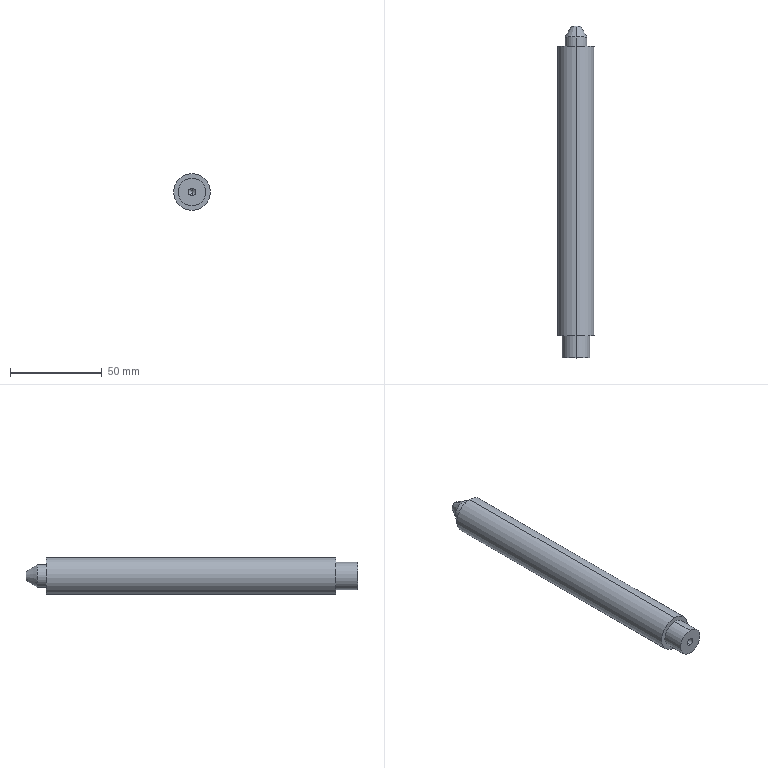Part | STEP file | 1 solid | 16 faces | box 20 x 181 x 20 mm | volume 52508 mm3 | cylinder 8 | cone 4 | plane 4 | commonest cylinder face diameters 4.2 x2 12 x2 15 x2 20 x2
STEP:
#1=CARTESIAN_POINT('',(0.,0.,0.));
#2=DIRECTION('',(0.,0.,1.));
#3=DIRECTION('',(1.,0.,0.));
#4=AXIS2_PLACEMENT_3D('',#1,#2,#3);
#5=CARTESIAN_POINT('',(0.,12.4,-2.1));
#6=VERTEX_POINT('',#5);
#7=CARTESIAN_POINT('',(0.,0.,-2.1));
#8=VERTEX_POINT('',#7);
#9=CARTESIAN_POINT('',(0.,0.,-2.1));
#10=DIRECTION('',(0.,-1.,0.));
#11=VECTOR('',#10,1.);
#12=LINE('',#9,#11);
#13=CARTESIAN_POINT('',(0.,0.,0.));
#14=DIRECTION('',(0.,-1.,0.));
#15=DIRECTION('',(0.,0.,-1.));
#16=AXIS2_PLACEMENT_3D('',#13,#14,#15);
#17=CYLINDRICAL_SURFACE('',#16,2.1);
#18=CARTESIAN_POINT('',(6.283,0.));
#19=DIRECTION('',(0.,1.));
#20=VECTOR('',#19,1.);
#21=LINE('',#18,#20);
#22=(GEOMETRIC_REPRESENTATION_CONTEXT(2)PARAMETRIC_REPRESENTATION_CONTEXT()REPRESENTATION_CONTEXT('',''));
#23=DEFINITIONAL_REPRESENTATION('',(#21),#22);
#24=PCURVE('',#17,#23);
#25=CARTESIAN_POINT('',(0.,0.,0.));
#26=DIRECTION('',(0.,-1.,0.));
#27=DIRECTION('',(0.,0.,-1.));
#28=AXIS2_PLACEMENT_3D('',#25,#26,#27);
#29=CYLINDRICAL_SURFACE('',#28,2.1);
#30=CARTESIAN_POINT('',(0.,0.));
#31=DIRECTION('',(0.,1.));
#32=VECTOR('',#31,1.);
#33=LINE('',#30,#32);
#34=(GEOMETRIC_REPRESENTATION_CONTEXT(2)PARAMETRIC_REPRESENTATION_CONTEXT()REPRESENTATION_CONTEXT('',''));
#35=DEFINITIONAL_REPRESENTATION('',(#33),#34);
#36=PCURVE('',#29,#35);
#37=SURFACE_CURVE('',#12,(#24,#36),.PCURVE_S1.);
#38=EDGE_CURVE('',#6,#8,#37,.T.);
#39=ORIENTED_EDGE('',*,*,#38,.T.);
#40=CARTESIAN_POINT('',(0.,0.,2.1));
#41=VERTEX_POINT('',#40);
#42=CARTESIAN_POINT('',(0.,0.,0.));
#43=DIRECTION('',(0.,-1.,0.));
#44=DIRECTION('',(0.,0.,-1.));
#45=AXIS2_PLACEMENT_3D('',#42,#43,#44);
#46=CIRCLE('',#45,2.1);
#47=CARTESIAN_POINT('',(0.,0.));
#48=DIRECTION('',(1.,0.));
#49=VECTOR('',#48,1.);
#50=LINE('',#47,#49);
#51=(GEOMETRIC_REPRESENTATION_CONTEXT(2)PARAMETRIC_REPRESENTATION_CONTEXT()REPRESENTATION_CONTEXT('',''));
#52=DEFINITIONAL_REPRESENTATION('',(#50),#51);
#53=PCURVE('',#17,#52);
#54=CARTESIAN_POINT('',(0.,0.,0.));
#55=DIRECTION('',(0.,-1.,0.));
#56=DIRECTION('',(0.,0.,-1.));
#57=AXIS2_PLACEMENT_3D('',#54,#55,#56);
#58=PLANE('',#57);
#59=CARTESIAN_POINT('',(0.,0.));
#60=DIRECTION('',(1.,0.));
#61=AXIS2_PLACEMENT_2D('',#59,#60);
#62=CIRCLE('',#61,2.1);
#63=(GEOMETRIC_REPRESENTATION_CONTEXT(2)PARAMETRIC_REPRESENTATION_CONTEXT()REPRESENTATION_CONTEXT('',''));
#64=DEFINITIONAL_REPRESENTATION('',(#62),#63);
#65=PCURVE('',#58,#64);
#66=SURFACE_CURVE('',#46,(#53,#65),.PCURVE_S1.);
#67=EDGE_CURVE('',#41,#8,#66,.T.);
#68=ORIENTED_EDGE('',*,*,#67,.F.);
#69=CARTESIAN_POINT('',(0.,12.4,2.1));
#70=VERTEX_POINT('',#69);
#71=CARTESIAN_POINT('',(0.,0.,2.1));
#72=DIRECTION('',(0.,-1.,0.));
#73=VECTOR('',#72,1.);
#74=LINE('',#71,#73);
#75=CARTESIAN_POINT('',(3.142,0.));
#76=DIRECTION('',(0.,1.));
#77=VECTOR('',#76,1.);
#78=LINE('',#75,#77);
#79=(GEOMETRIC_REPRESENTATION_CONTEXT(2)PARAMETRIC_REPRESENTATION_CONTEXT()REPRESENTATION_CONTEXT('',''));
#80=DEFINITIONAL_REPRESENTATION('',(#78),#79);
#81=PCURVE('',#17,#80);
#82=CARTESIAN_POINT('',(3.142,0.));
#83=DIRECTION('',(0.,1.));
#84=VECTOR('',#83,1.);
#85=LINE('',#82,#84);
#86=(GEOMETRIC_REPRESENTATION_CONTEXT(2)PARAMETRIC_REPRESENTATION_CONTEXT()REPRESENTATION_CONTEXT('',''));
#87=DEFINITIONAL_REPRESENTATION('',(#85),#86);
#88=PCURVE('',#29,#87);
#89=SURFACE_CURVE('',#74,(#81,#88),.PCURVE_S1.);
#90=EDGE_CURVE('',#70,#41,#89,.T.);
#91=ORIENTED_EDGE('',*,*,#90,.F.);
#92=CARTESIAN_POINT('',(0.,12.4,0.));
#93=DIRECTION('',(0.,-1.,0.));
#94=DIRECTION('',(0.,0.,-1.));
#95=AXIS2_PLACEMENT_3D('',#92,#93,#94);
#96=CIRCLE('',#95,2.1);
#97=CARTESIAN_POINT('',(0.,-12.4));
#98=DIRECTION('',(1.,0.));
#99=VECTOR('',#98,1.);
#100=LINE('',#97,#99);
#101=(GEOMETRIC_REPRESENTATION_CONTEXT(2)PARAMETRIC_REPRESENTATION_CONTEXT()REPRESENTATION_CONTEXT('',''));
#102=DEFINITIONAL_REPRESENTATION('',(#100),#101);
#103=PCURVE('',#17,#102);
#104=CARTESIAN_POINT('',(0.,12.4,0.));
#105=DIRECTION('',(0.,-1.,0.));
#106=DIRECTION('',(0.,0.,-1.));
#107=AXIS2_PLACEMENT_3D('',#104,#105,#106);
#108=CONICAL_SURFACE('',#107,2.1,1.03);
#109=CARTESIAN_POINT('',(0.,0.));
#110=DIRECTION('',(1.,0.));
#111=VECTOR('',#110,1.);
#112=LINE('',#109,#111);
#113=(GEOMETRIC_REPRESENTATION_CONTEXT(2)PARAMETRIC_REPRESENTATION_CONTEXT()REPRESENTATION_CONTEXT('',''));
#114=DEFINITIONAL_REPRESENTATION('',(#112),#113);
#115=PCURVE('',#108,#114);
#116=SURFACE_CURVE('',#96,(#103,#115),.PCURVE_S1.);
#117=EDGE_CURVE('',#70,#6,#116,.T.);
#118=ORIENTED_EDGE('',*,*,#117,.T.);
#119=EDGE_LOOP('',(#39,#68,#91,#118));
#120=FACE_BOUND('',#119,.F.);
#121=ADVANCED_FACE('',(#120),#17,.F.);
#122=ORIENTED_EDGE('',*,*,#117,.F.);
#123=CARTESIAN_POINT('',(0.,13.662,0.));
#124=VERTEX_POINT('',#123);
#125=CARTESIAN_POINT('',(0.,12.4,2.1));
#126=DIRECTION('',(0.,-0.515,0.8572));
#127=VECTOR('',#126,1.);
#128=LINE('',#125,#127);
#129=CARTESIAN_POINT('',(3.142,0.));
#130=DIRECTION('',(0.,1.));
#131=VECTOR('',#130,1.);
#132=LINE('',#129,#131);
#133=(GEOMETRIC_REPRESENTATION_CONTEXT(2)PARAMETRIC_REPRESENTATION_CONTEXT()REPRESENTATION_CONTEXT('',''));
#134=DEFINITIONAL_REPRESENTATION('',(#132),#133);
#135=PCURVE('',#108,#134);
#136=CARTESIAN_POINT('',(0.,12.4,0.));
#137=DIRECTION('',(0.,-1.,0.));
#138=DIRECTION('',(0.,0.,-1.));
#139=AXIS2_PLACEMENT_3D('',#136,#137,#138);
#140=CONICAL_SURFACE('',#139,2.1,1.03);
#141=CARTESIAN_POINT('',(3.142,0.));
#142=DIRECTION('',(0.,1.));
#143=VECTOR('',#142,1.);
#144=LINE('',#141,#143);
#145=(GEOMETRIC_REPRESENTATION_CONTEXT(2)PARAMETRIC_REPRESENTATION_CONTEXT()REPRESENTATION_CONTEXT('',''));
#146=DEFINITIONAL_REPRESENTATION('',(#144),#145);
#147=PCURVE('',#140,#146);
#148=SURFACE_CURVE('',#128,(#135,#147),.PCURVE_S1.);
#149=EDGE_CURVE('',#124,#70,#148,.T.);
#150=ORIENTED_EDGE('',*,*,#149,.F.);
#151=CARTESIAN_POINT('',(0.,12.4,-2.1));
#152=DIRECTION('',(0.,-0.515,-0.8572));
#153=VECTOR('',#152,1.);
#154=LINE('',#151,#153);
#155=CARTESIAN_POINT('',(6.283,0.));
#156=DIRECTION('',(0.,1.));
#157=VECTOR('',#156,1.);
#158=LINE('',#155,#157);
#159=(GEOMETRIC_REPRESENTATION_CONTEXT(2)PARAMETRIC_REPRESENTATION_CONTEXT()REPRESENTATION_CONTEXT('',''));
#160=DEFINITIONAL_REPRESENTATION('',(#158),#159);
#161=PCURVE('',#108,#160);
#162=CARTESIAN_POINT('',(0.,0.));
#163=DIRECTION('',(0.,1.));
#164=VECTOR('',#163,1.);
#165=LINE('',#162,#164);
#166=(GEOMETRIC_REPRESENTATION_CONTEXT(2)PARAMETRIC_REPRESENTATION_CONTEXT()REPRESENTATION_CONTEXT('',''));
#167=DEFINITIONAL_REPRESENTATION('',(#165),#166);
#168=PCURVE('',#140,#167);
#169=SURFACE_CURVE('',#154,(#161,#168),.PCURVE_S1.);
#170=EDGE_CURVE('',#124,#6,#169,.T.);
#171=ORIENTED_EDGE('',*,*,#170,.T.);
#172=EDGE_LOOP('',(#122,#150,#171));
#173=FACE_BOUND('',#172,.F.);
#174=ADVANCED_FACE('',(#173),#108,.F.);
#175=CARTESIAN_POINT('',(0.,181.,-2.536));
#176=VERTEX_POINT('',#175);
#177=CARTESIAN_POINT('',(0.,181.,2.536));
#178=VERTEX_POINT('',#177);
#179=CARTESIAN_POINT('',(0.,181.,0.));
#180=DIRECTION('',(0.,-1.,0.));
#181=DIRECTION('',(0.,0.,-1.));
#182=AXIS2_PLACEMENT_3D('',#179,#180,#181);
#183=CIRCLE('',#182,2.536);
#184=CARTESIAN_POINT('',(0.,175.,0.));
#185=DIRECTION('',(0.,-1.,0.));
#186=DIRECTION('',(0.,0.,-1.));
#187=AXIS2_PLACEMENT_3D('',#184,#185,#186);
#188=CONICAL_SURFACE('',#187,6.,0.5236);
#189=CARTESIAN_POINT('',(0.,-6.));
#190=DIRECTION('',(1.,0.));
#191=VECTOR('',#190,1.);
#192=LINE('',#189,#191);
#193=(GEOMETRIC_REPRESENTATION_CONTEXT(2)PARAMETRIC_REPRESENTATION_CONTEXT()REPRESENTATION_CONTEXT('',''));
#194=DEFINITIONAL_REPRESENTATION('',(#192),#193);
#195=PCURVE('',#188,#194);
#196=CARTESIAN_POINT('',(2.536,181.,0.));
#197=DIRECTION('',(0.,1.,0.));
#198=DIRECTION('',(0.,0.,1.));
#199=AXIS2_PLACEMENT_3D('',#196,#197,#198);
#200=PLANE('',#199);
#201=CARTESIAN_POINT('',(-2.536,-2.536));
#202=CARTESIAN_POINT('',(-2.536,1.856));
#203=CARTESIAN_POINT('',(1.268,-0.3397));
#204=CARTESIAN_POINT('',(5.072,-2.536));
#205=CARTESIAN_POINT('',(1.268,-4.732));
#206=CARTESIAN_POINT('',(-2.536,-6.928));
#207=CARTESIAN_POINT('',(-2.536,-2.536));
#208=(BOUNDED_CURVE()B_SPLINE_CURVE(2,(#201,#202,#203,#204,#205,#206,#207),.UNSPECIFIED.,.T.,.F.)B_SPLINE_CURVE_WITH_KNOTS((1,2,2,2,2,1),(-2.094,0.,2.094,4.189,6.283,8.378),.UNSPECIFIED.)CURVE()GEOMETRIC_REPRESENTATION_ITEM()RATIONAL_B_SPLINE_CURVE((1.,0.5,1.,0.5,1.,0.5,1.))REPRESENTATION_ITEM(''));
#209=(GEOMETRIC_REPRESENTATION_CONTEXT(2)PARAMETRIC_REPRESENTATION_CONTEXT()REPRESENTATION_CONTEXT('',''));
#210=DEFINITIONAL_REPRESENTATION('',(#208),#209);
#211=PCURVE('',#200,#210);
#212=SURFACE_CURVE('',#183,(#195,#211),.PCURVE_S1.);
#213=EDGE_CURVE('',#176,#178,#212,.T.);
#214=ORIENTED_EDGE('',*,*,#213,.T.);
#215=CARTESIAN_POINT('',(0.,175.,6.));
#216=VERTEX_POINT('',#215);
#217=CARTESIAN_POINT('',(0.,175.,6.));
#218=DIRECTION('',(0.,-0.866,0.5));
#219=VECTOR('',#218,1.);
#220=LINE('',#217,#219);
#221=CARTESIAN_POINT('',(3.142,0.));
#222=DIRECTION('',(0.,1.));
#223=VECTOR('',#222,1.);
#224=LINE('',#221,#223);
#225=(GEOMETRIC_REPRESENTATION_CONTEXT(2)PARAMETRIC_REPRESENTATION_CONTEXT()REPRESENTATION_CONTEXT('',''));
#226=DEFINITIONAL_REPRESENTATION('',(#224),#225);
#227=PCURVE('',#188,#226);
#228=CARTESIAN_POINT('',(0.,175.,0.));
#229=DIRECTION('',(0.,-1.,0.));
#230=DIRECTION('',(0.,0.,-1.));
#231=AXIS2_PLACEMENT_3D('',#228,#229,#230);
#232=CONICAL_SURFACE('',#231,6.,0.5236);
#233=CARTESIAN_POINT('',(3.142,0.));
#234=DIRECTION('',(0.,1.));
#235=VECTOR('',#234,1.);
#236=LINE('',#233,#235);
#237=(GEOMETRIC_REPRESENTATION_CONTEXT(2)PARAMETRIC_REPRESENTATION_CONTEXT()REPRESENTATION_CONTEXT('',''));
#238=DEFINITIONAL_REPRESENTATION('',(#236),#237);
#239=PCURVE('',#232,#238);
#240=SURFACE_CURVE('',#220,(#227,#239),.PCURVE_S1.);
#241=EDGE_CURVE('',#178,#216,#240,.T.);
#242=ORIENTED_EDGE('',*,*,#241,.T.);
#243=CARTESIAN_POINT('',(0.,175.,-6.));
#244=VERTEX_POINT('',#243);
#245=CARTESIAN_POINT('',(0.,175.,0.));
#246=DIRECTION('',(0.,-1.,0.));
#247=DIRECTION('',(0.,0.,-1.));
#248=AXIS2_PLACEMENT_3D('',#245,#246,#247);
#249=CIRCLE('',#248,6.);
#250=CARTESIAN_POINT('',(0.,0.));
#251=DIRECTION('',(1.,0.));
#252=VECTOR('',#251,1.);
#253=LINE('',#250,#252);
#254=(GEOMETRIC_REPRESENTATION_CONTEXT(2)PARAMETRIC_REPRESENTATION_CONTEXT()REPRESENTATION_CONTEXT('',''));
#255=DEFINITIONAL_REPRESENTATION('',(#253),#254);
#256=PCURVE('',#188,#255);
#257=CARTESIAN_POINT('',(0.,0.,0.));
#258=DIRECTION('',(0.,-1.,0.));
#259=DIRECTION('',(0.,0.,-1.));
#260=AXIS2_PLACEMENT_3D('',#257,#258,#259);
#261=CYLINDRICAL_SURFACE('',#260,6.);
#262=CARTESIAN_POINT('',(0.,-175.));
#263=DIRECTION('',(1.,0.));
#264=VECTOR('',#263,1.);
#265=LINE('',#262,#264);
#266=(GEOMETRIC_REPRESENTATION_CONTEXT(2)PARAMETRIC_REPRESENTATION_CONTEXT()REPRESENTATION_CONTEXT('',''));
#267=DEFINITIONAL_REPRESENTATION('',(#265),#266);
#268=PCURVE('',#261,#267);
#269=SURFACE_CURVE('',#249,(#256,#268),.PCURVE_S1.);
#270=EDGE_CURVE('',#244,#216,#269,.T.);
#271=ORIENTED_EDGE('',*,*,#270,.F.);
#272=CARTESIAN_POINT('',(0.,175.,-6.));
#273=DIRECTION('',(0.,-0.866,-0.5));
#274=VECTOR('',#273,1.);
#275=LINE('',#272,#274);
#276=CARTESIAN_POINT('',(0.,0.));
#277=DIRECTION('',(0.,1.));
#278=VECTOR('',#277,1.);
#279=LINE('',#276,#278);
#280=(GEOMETRIC_REPRESENTATION_CONTEXT(2)PARAMETRIC_REPRESENTATION_CONTEXT()REPRESENTATION_CONTEXT('',''));
#281=DEFINITIONAL_REPRESENTATION('',(#279),#280);
#282=PCURVE('',#188,#281);
#283=CARTESIAN_POINT('',(6.283,0.));
#284=DIRECTION('',(0.,1.));
#285=VECTOR('',#284,1.);
#286=LINE('',#283,#285);
#287=(GEOMETRIC_REPRESENTATION_CONTEXT(2)PARAMETRIC_REPRESENTATION_CONTEXT()REPRESENTATION_CONTEXT('',''));
#288=DEFINITIONAL_REPRESENTATION('',(#286),#287);
#289=PCURVE('',#232,#288);
#290=SURFACE_CURVE('',#275,(#282,#289),.PCURVE_S1.);
#291=EDGE_CURVE('',#176,#244,#290,.T.);
#292=ORIENTED_EDGE('',*,*,#291,.F.);
#293=EDGE_LOOP('',(#214,#242,#271,#292));
#294=FACE_BOUND('',#293,.T.);
#295=ADVANCED_FACE('',(#294),#188,.T.);
#296=ORIENTED_EDGE('',*,*,#270,.T.);
#297=CARTESIAN_POINT('',(0.,170.,6.));
#298=VERTEX_POINT('',#297);
#299=CARTESIAN_POINT('',(0.,0.,6.));
#300=DIRECTION('',(0.,-1.,0.));
#301=VECTOR('',#300,1.);
#302=LINE('',#299,#301);
#303=CARTESIAN_POINT('',(3.142,0.));
#304=DIRECTION('',(0.,1.));
#305=VECTOR('',#304,1.);
#306=LINE('',#303,#305);
#307=(GEOMETRIC_REPRESENTATION_CONTEXT(2)PARAMETRIC_REPRESENTATION_CONTEXT()REPRESENTATION_CONTEXT('',''));
#308=DEFINITIONAL_REPRESENTATION('',(#306),#307);
#309=PCURVE('',#261,#308);
#310=CARTESIAN_POINT('',(0.,0.,0.));
#311=DIRECTION('',(0.,-1.,0.));
#312=DIRECTION('',(0.,0.,-1.));
#313=AXIS2_PLACEMENT_3D('',#310,#311,#312);
#314=CYLINDRICAL_SURFACE('',#313,6.);
#315=CARTESIAN_POINT('',(3.142,0.));
#316=DIRECTION('',(0.,1.));
#317=VECTOR('',#316,1.);
#318=LINE('',#315,#317);
#319=(GEOMETRIC_REPRESENTATION_CONTEXT(2)PARAMETRIC_REPRESENTATION_CONTEXT()REPRESENTATION_CONTEXT('',''));
#320=DEFINITIONAL_REPRESENTATION('',(#318),#319);
#321=PCURVE('',#314,#320);
#322=SURFACE_CURVE('',#302,(#309,#321),.PCURVE_S1.);
#323=EDGE_CURVE('',#216,#298,#322,.T.);
#324=ORIENTED_EDGE('',*,*,#323,.T.);
#325=CARTESIAN_POINT('',(0.,170.,-6.));
#326=VERTEX_POINT('',#325);
#327=CARTESIAN_POINT('',(0.,170.,0.));
#328=DIRECTION('',(0.,-1.,0.));
#329=DIRECTION('',(0.,0.,-1.));
#330=AXIS2_PLACEMENT_3D('',#327,#328,#329);
#331=CIRCLE('',#330,6.);
#332=CARTESIAN_POINT('',(0.,-170.));
#333=DIRECTION('',(1.,0.));
#334=VECTOR('',#333,1.);
#335=LINE('',#332,#334);
#336=(GEOMETRIC_REPRESENTATION_CONTEXT(2)PARAMETRIC_REPRESENTATION_CONTEXT()REPRESENTATION_CONTEXT('',''));
#337=DEFINITIONAL_REPRESENTATION('',(#335),#336);
#338=PCURVE('',#261,#337);
#339=CARTESIAN_POINT('',(10.,170.,0.));
#340=DIRECTION('',(0.,1.,0.));
#341=DIRECTION('',(0.,0.,1.));
#342=AXIS2_PLACEMENT_3D('',#339,#340,#341);
#343=PLANE('',#342);
#344=CARTESIAN_POINT('',(-6.,-10.));
#345=CARTESIAN_POINT('',(-6.,0.3923));
#346=CARTESIAN_POINT('',(3.,-4.804));
#347=CARTESIAN_POINT('',(12.,-10.));
#348=CARTESIAN_POINT('',(3.,-15.196));
#349=CARTESIAN_POINT('',(-6.,-20.392));
#350=CARTESIAN_POINT('',(-6.,-10.));
#351=(BOUNDED_CURVE()B_SPLINE_CURVE(2,(#344,#345,#346,#347,#348,#349,#350),.UNSPECIFIED.,.T.,.F.)B_SPLINE_CURVE_WITH_KNOTS((1,2,2,2,2,1),(-2.094,0.,2.094,4.189,6.283,8.378),.UNSPECIFIED.)CURVE()GEOMETRIC_REPRESENTATION_ITEM()RATIONAL_B_SPLINE_CURVE((1.,0.5,1.,0.5,1.,0.5,1.))REPRESENTATION_ITEM(''));
#352=(GEOMETRIC_REPRESENTATION_CONTEXT(2)PARAMETRIC_REPRESENTATION_CONTEXT()REPRESENTATION_CONTEXT('',''));
#353=DEFINITIONAL_REPRESENTATION('',(#351),#352);
#354=PCURVE('',#343,#353);
#355=SURFACE_CURVE('',#331,(#338,#354),.PCURVE_S1.);
#356=EDGE_CURVE('',#326,#298,#355,.T.);
#357=ORIENTED_EDGE('',*,*,#356,.F.);
#358=CARTESIAN_POINT('',(0.,0.,-6.));
#359=DIRECTION('',(0.,-1.,0.));
#360=VECTOR('',#359,1.);
#361=LINE('',#358,#360);
#362=CARTESIAN_POINT('',(0.,0.));
#363=DIRECTION('',(0.,1.));
#364=VECTOR('',#363,1.);
#365=LINE('',#362,#364);
#366=(GEOMETRIC_REPRESENTATION_CONTEXT(2)PARAMETRIC_REPRESENTATION_CONTEXT()REPRESENTATION_CONTEXT('',''));
#367=DEFINITIONAL_REPRESENTATION('',(#365),#366);
#368=PCURVE('',#261,#367);
#369=CARTESIAN_POINT('',(6.283,0.));
#370=DIRECTION('',(0.,1.));
#371=VECTOR('',#370,1.);
#372=LINE('',#369,#371);
#373=(GEOMETRIC_REPRESENTATION_CONTEXT(2)PARAMETRIC_REPRESENTATION_CONTEXT()REPRESENTATION_CONTEXT('',''));
#374=DEFINITIONAL_REPRESENTATION('',(#372),#373);
#375=PCURVE('',#314,#374);
#376=SURFACE_CURVE('',#361,(#368,#375),.PCURVE_S1.);
#377=EDGE_CURVE('',#244,#326,#376,.T.);
#378=ORIENTED_EDGE('',*,*,#377,.F.);
#379=EDGE_LOOP('',(#296,#324,#357,#378));
#380=FACE_BOUND('',#379,.T.);
#381=ADVANCED_FACE('',(#380),#261,.T.);
#382=CARTESIAN_POINT('',(0.,170.,-10.));
#383=VERTEX_POINT('',#382);
#384=CARTESIAN_POINT('',(0.,170.,10.));
#385=VERTEX_POINT('',#384);
#386=CARTESIAN_POINT('',(0.,170.,0.));
#387=DIRECTION('',(0.,-1.,0.));
#388=DIRECTION('',(0.,0.,-1.));
#389=AXIS2_PLACEMENT_3D('',#386,#387,#388);
#390=CIRCLE('',#389,10.);
#391=CARTESIAN_POINT('',(0.,0.,0.));
#392=DIRECTION('',(0.,-1.,0.));
#393=DIRECTION('',(0.,0.,-1.));
#394=AXIS2_PLACEMENT_3D('',#391,#392,#393);
#395=CYLINDRICAL_SURFACE('',#394,10.);
#396=CARTESIAN_POINT('',(0.,-170.));
#397=DIRECTION('',(1.,0.));
#398=VECTOR('',#397,1.);
#399=LINE('',#396,#398);
#400=(GEOMETRIC_REPRESENTATION_CONTEXT(2)PARAMETRIC_REPRESENTATION_CONTEXT()REPRESENTATION_CONTEXT('',''));
#401=DEFINITIONAL_REPRESENTATION('',(#399),#400);
#402=PCURVE('',#395,#401);
#403=CARTESIAN_POINT('',(-10.,-10.));
#404=CARTESIAN_POINT('',(-10.,7.321));
#405=CARTESIAN_POINT('',(5.,-1.34));
#406=CARTESIAN_POINT('',(20.,-10.));
#407=CARTESIAN_POINT('',(5.,-18.66));
#408=CARTESIAN_POINT('',(-10.,-27.321));
#409=CARTESIAN_POINT('',(-10.,-10.));
#410=(BOUNDED_CURVE()B_SPLINE_CURVE(2,(#403,#404,#405,#406,#407,#408,#409),.UNSPECIFIED.,.T.,.F.)B_SPLINE_CURVE_WITH_KNOTS((1,2,2,2,2,1),(-2.094,0.,2.094,4.189,6.283,8.378),.UNSPECIFIED.)CURVE()GEOMETRIC_REPRESENTATION_ITEM()RATIONAL_B_SPLINE_CURVE((1.,0.5,1.,0.5,1.,0.5,1.))REPRESENTATION_ITEM(''));
#411=(GEOMETRIC_REPRESENTATION_CONTEXT(2)PARAMETRIC_REPRESENTATION_CONTEXT()REPRESENTATION_CONTEXT('',''));
#412=DEFINITIONAL_REPRESENTATION('',(#410),#411);
#413=PCURVE('',#343,#412);
#414=SURFACE_CURVE('',#390,(#402,#413),.PCURVE_S1.);
#415=EDGE_CURVE('',#383,#385,#414,.T.);
#416=ORIENTED_EDGE('',*,*,#415,.T.);
#417=CARTESIAN_POINT('',(0.,12.,10.));
#418=VERTEX_POINT('',#417);
#419=CARTESIAN_POINT('',(0.,0.,10.));
#420=DIRECTION('',(0.,-1.,0.));
#421=VECTOR('',#420,1.);
#422=LINE('',#419,#421);
#423=CARTESIAN_POINT('',(3.142,0.));
#424=DIRECTION('',(0.,1.));
#425=VECTOR('',#424,1.);
#426=LINE('',#423,#425);
#427=(GEOMETRIC_REPRESENTATION_CONTEXT(2)PARAMETRIC_REPRESENTATION_CONTEXT()REPRESENTATION_CONTEXT('',''));
#428=DEFINITIONAL_REPRESENTATION('',(#426),#427);
#429=PCURVE('',#395,#428);
#430=CARTESIAN_POINT('',(0.,0.,0.));
#431=DIRECTION('',(0.,-1.,0.));
#432=DIRECTION('',(0.,0.,-1.));
#433=AXIS2_PLACEMENT_3D('',#430,#431,#432);
#434=CYLINDRICAL_SURFACE('',#433,10.);
#435=CARTESIAN_POINT('',(3.142,0.));
#436=DIRECTION('',(0.,1.));
#437=VECTOR('',#436,1.);
#438=LINE('',#435,#437);
#439=(GEOMETRIC_REPRESENTATION_CONTEXT(2)PARAMETRIC_REPRESENTATION_CONTEXT()REPRESENTATION_CONTEXT('',''));
#440=DEFINITIONAL_REPRESENTATION('',(#438),#439);
#441=PCURVE('',#434,#440);
#442=SURFACE_CURVE('',#422,(#429,#441),.PCURVE_S1.);
#443=EDGE_CURVE('',#385,#418,#442,.T.);
#444=ORIENTED_EDGE('',*,*,#443,.T.);
#445=CARTESIAN_POINT('',(0.,12.,-10.));
#446=VERTEX_POINT('',#445);
#447=CARTESIAN_POINT('',(0.,12.,0.));
#448=DIRECTION('',(0.,-1.,0.));
#449=DIRECTION('',(0.,0.,-1.));
#450=AXIS2_PLACEMENT_3D('',#447,#448,#449);
#451=CIRCLE('',#450,10.);
#452=CARTESIAN_POINT('',(0.,-12.));
#453=DIRECTION('',(1.,0.));
#454=VECTOR('',#453,1.);
#455=LINE('',#452,#454);
#456=(GEOMETRIC_REPRESENTATION_CONTEXT(2)PARAMETRIC_REPRESENTATION_CONTEXT()REPRESENTATION_CONTEXT('',''));
#457=DEFINITIONAL_REPRESENTATION('',(#455),#456);
#458=PCURVE('',#395,#457);
#459=CARTESIAN_POINT('',(7.5,12.,0.));
#460=DIRECTION('',(0.,-1.,0.));
#461=DIRECTION('',(0.,0.,-1.));
#462=AXIS2_PLACEMENT_3D('',#459,#460,#461);
#463=PLANE('',#462);
#464=CARTESIAN_POINT('',(0.,-7.5));
#465=DIRECTION('',(1.,0.));
#466=AXIS2_PLACEMENT_2D('',#464,#465);
#467=CIRCLE('',#466,10.);
#468=(GEOMETRIC_REPRESENTATION_CONTEXT(2)PARAMETRIC_REPRESENTATION_CONTEXT()REPRESENTATION_CONTEXT('',''));
#469=DEFINITIONAL_REPRESENTATION('',(#467),#468);
#470=PCURVE('',#463,#469);
#471=SURFACE_CURVE('',#451,(#458,#470),.PCURVE_S1.);
#472=EDGE_CURVE('',#446,#418,#471,.T.);
#473=ORIENTED_EDGE('',*,*,#472,.F.);
#474=CARTESIAN_POINT('',(0.,0.,-10.));
#475=DIRECTION('',(0.,-1.,0.));
#476=VECTOR('',#475,1.);
#477=LINE('',#474,#476);
#478=CARTESIAN_POINT('',(0.,0.));
#479=DIRECTION('',(0.,1.));
#480=VECTOR('',#479,1.);
#481=LINE('',#478,#480);
#482=(GEOMETRIC_REPRESENTATION_CONTEXT(2)PARAMETRIC_REPRESENTATION_CONTEXT()REPRESENTATION_CONTEXT('',''));
#483=DEFINITIONAL_REPRESENTATION('',(#481),#482);
#484=PCURVE('',#395,#483);
#485=CARTESIAN_POINT('',(6.283,0.));
#486=DIRECTION('',(0.,1.));
#487=VECTOR('',#486,1.);
#488=LINE('',#485,#487);
#489=(GEOMETRIC_REPRESENTATION_CONTEXT(2)PARAMETRIC_REPRESENTATION_CONTEXT()REPRESENTATION_CONTEXT('',''));
#490=DEFINITIONAL_REPRESENTATION('',(#488),#489);
#491=PCURVE('',#434,#490);
#492=SURFACE_CURVE('',#477,(#484,#491),.PCURVE_S1.);
#493=EDGE_CURVE('',#383,#446,#492,.T.);
#494=ORIENTED_EDGE('',*,*,#493,.F.);
#495=EDGE_LOOP('',(#416,#444,#473,#494));
#496=FACE_BOUND('',#495,.T.);
#497=ADVANCED_FACE('',(#496),#395,.T.);
#498=CARTESIAN_POINT('',(0.,12.,-7.5));
#499=VERTEX_POINT('',#498);
#500=CARTESIAN_POINT('',(0.,12.,7.5));
#501=VERTEX_POINT('',#500);
#502=CARTESIAN_POINT('',(0.,12.,0.));
#503=DIRECTION('',(0.,-1.,0.));
#504=DIRECTION('',(0.,0.,-1.));
#505=AXIS2_PLACEMENT_3D('',#502,#503,#504);
#506=CIRCLE('',#505,7.5);
#507=CARTESIAN_POINT('',(0.,0.,0.));
#508=DIRECTION('',(0.,-1.,0.));
#509=DIRECTION('',(0.,0.,-1.));
#510=AXIS2_PLACEMENT_3D('',#507,#508,#509);
#511=CYLINDRICAL_SURFACE('',#510,7.5);
#512=CARTESIAN_POINT('',(0.,-12.));
#513=DIRECTION('',(1.,0.));
#514=VECTOR('',#513,1.);
#515=LINE('',#512,#514);
#516=(GEOMETRIC_REPRESENTATION_CONTEXT(2)PARAMETRIC_REPRESENTATION_CONTEXT()REPRESENTATION_CONTEXT('',''));
#517=DEFINITIONAL_REPRESENTATION('',(#515),#516);
#518=PCURVE('',#511,#517);
#519=CARTESIAN_POINT('',(0.,-7.5));
#520=DIRECTION('',(1.,0.));
#521=AXIS2_PLACEMENT_2D('',#519,#520);
#522=CIRCLE('',#521,7.5);
#523=(GEOMETRIC_REPRESENTATION_CONTEXT(2)PARAMETRIC_REPRESENTATION_CONTEXT()REPRESENTATION_CONTEXT('',''));
#524=DEFINITIONAL_REPRESENTATION('',(#522),#523);
#525=PCURVE('',#463,#524);
#526=SURFACE_CURVE('',#506,(#518,#525),.PCURVE_S1.);
#527=EDGE_CURVE('',#499,#501,#526,.T.);
#528=ORIENTED_EDGE('',*,*,#527,.T.);
#529=CARTESIAN_POINT('',(0.,0.,7.5));
#530=VERTEX_POINT('',#529);
#531=CARTESIAN_POINT('',(0.,0.,7.5));
#532=DIRECTION('',(0.,-1.,0.));
#533=VECTOR('',#532,1.);
#534=LINE('',#531,#533);
#535=CARTESIAN_POINT('',(3.142,0.));
#536=DIRECTION('',(0.,1.));
#537=VECTOR('',#536,1.);
#538=LINE('',#535,#537);
#539=(GEOMETRIC_REPRESENTATION_CONTEXT(2)PARAMETRIC_REPRESENTATION_CONTEXT()REPRESENTATION_CONTEXT('',''));
#540=DEFINITIONAL_REPRESENTATION('',(#538),#539);
#541=PCURVE('',#511,#540);
#542=CARTESIAN_POINT('',(0.,0.,0.));
#543=DIRECTION('',(0.,-1.,0.));
#544=DIRECTION('',(0.,0.,-1.));
#545=AXIS2_PLACEMENT_3D('',#542,#543,#544);
#546=CYLINDRICAL_SURFACE('',#545,7.5);
#547=CARTESIAN_POINT('',(3.142,0.));
#548=DIRECTION('',(0.,1.));
#549=VECTOR('',#548,1.);
#550=LINE('',#547,#549);
#551=(GEOMETRIC_REPRESENTATION_CONTEXT(2)PARAMETRIC_REPRESENTATION_CONTEXT()REPRESENTATION_CONTEXT('',''));
#552=DEFINITIONAL_REPRESENTATION('',(#550),#551);
#553=PCURVE('',#546,#552);
#554=SURFACE_CURVE('',#534,(#541,#553),.PCURVE_S1.);
#555=EDGE_CURVE('',#501,#530,#554,.T.);
#556=ORIENTED_EDGE('',*,*,#555,.T.);
#557=CARTESIAN_POINT('',(0.,0.,-7.5));
#558=VERTEX_POINT('',#557);
#559=CARTESIAN_POINT('',(0.,0.,0.));
#560=DIRECTION('',(0.,-1.,0.));
#561=DIRECTION('',(0.,0.,-1.));
#562=AXIS2_PLACEMENT_3D('',#559,#560,#561);
#563=CIRCLE('',#562,7.5);
#564=CARTESIAN_POINT('',(0.,0.));
#565=DIRECTION('',(1.,0.));
#566=VECTOR('',#565,1.);
#567=LINE('',#564,#566);
#568=(GEOMETRIC_REPRESENTATION_CONTEXT(2)PARAMETRIC_REPRESENTATION_CONTEXT()REPRESENTATION_CONTEXT('',''));
#569=DEFINITIONAL_REPRESENTATION('',(#567),#568);
#570=PCURVE('',#511,#569);
#571=CARTESIAN_POINT('',(0.,0.));
#572=DIRECTION('',(1.,0.));
#573=AXIS2_PLACEMENT_2D('',#571,#572);
#574=CIRCLE('',#573,7.5);
#575=(GEOMETRIC_REPRESENTATION_CONTEXT(2)PARAMETRIC_REPRESENTATION_CONTEXT()REPRESENTATION_CONTEXT('',''));
#576=DEFINITIONAL_REPRESENTATION('',(#574),#575);
#577=PCURVE('',#58,#576);
#578=SURFACE_CURVE('',#563,(#570,#577),.PCURVE_S1.);
#579=EDGE_CURVE('',#558,#530,#578,.T.);
#580=ORIENTED_EDGE('',*,*,#579,.F.);
#581=CARTESIAN_POINT('',(0.,0.,-7.5));
#582=DIRECTION('',(0.,-1.,0.));
#583=VECTOR('',#582,1.);
#584=LINE('',#581,#583);
#585=CARTESIAN_POINT('',(0.,0.));
#586=DIRECTION('',(0.,1.));
#587=VECTOR('',#586,1.);
#588=LINE('',#585,#587);
#589=(GEOMETRIC_REPRESENTATION_CONTEXT(2)PARAMETRIC_REPRESENTATION_CONTEXT()REPRESENTATION_CONTEXT('',''));
#590=DEFINITIONAL_REPRESENTATION('',(#588),#589);
#591=PCURVE('',#511,#590);
#592=CARTESIAN_POINT('',(6.283,0.));
#593=DIRECTION('',(0.,1.));
#594=VECTOR('',#593,1.);
#595=LINE('',#592,#594);
#596=(GEOMETRIC_REPRESENTATION_CONTEXT(2)PARAMETRIC_REPRESENTATION_CONTEXT()REPRESENTATION_CONTEXT('',''));
#597=DEFINITIONAL_REPRESENTATION('',(#595),#596);
#598=PCURVE('',#546,#597);
#599=SURFACE_CURVE('',#584,(#591,#598),.PCURVE_S1.);
#600=EDGE_CURVE('',#499,#558,#599,.T.);
#601=ORIENTED_EDGE('',*,*,#600,.F.);
#602=EDGE_LOOP('',(#528,#556,#580,#601));
#603=FACE_BOUND('',#602,.T.);
#604=ADVANCED_FACE('',(#603),#511,.T.);
#605=CARTESIAN_POINT('',(0.,0.,0.));
#606=DIRECTION('',(0.,-1.,0.));
#607=DIRECTION('',(0.,0.,-1.));
#608=AXIS2_PLACEMENT_3D('',#605,#606,#607);
#609=CIRCLE('',#608,2.1);
#610=CARTESIAN_POINT('',(0.,0.));
#611=DIRECTION('',(1.,0.));
#612=AXIS2_PLACEMENT_2D('',#610,#611);
#613=CIRCLE('',#612,2.1);
#614=(GEOMETRIC_REPRESENTATION_CONTEXT(2)PARAMETRIC_REPRESENTATION_CONTEXT()REPRESENTATION_CONTEXT('',''));
#615=DEFINITIONAL_REPRESENTATION('',(#613),#614);
#616=PCURVE('',#58,#615);
#617=CARTESIAN_POINT('',(0.,0.));
#618=DIRECTION('',(1.,0.));
#619=VECTOR('',#618,1.);
#620=LINE('',#617,#619);
#621=(GEOMETRIC_REPRESENTATION_CONTEXT(2)PARAMETRIC_REPRESENTATION_CONTEXT()REPRESENTATION_CONTEXT('',''));
#622=DEFINITIONAL_REPRESENTATION('',(#620),#621);
#623=PCURVE('',#29,#622);
#624=SURFACE_CURVE('',#609,(#616,#623),.PCURVE_S1.);
#625=EDGE_CURVE('',#8,#41,#624,.T.);
#626=ORIENTED_EDGE('',*,*,#625,.F.);
#627=ORIENTED_EDGE('',*,*,#67,.F.);
#628=EDGE_LOOP('',(#626,#627));
#629=FACE_BOUND('',#628,.T.);
#630=ORIENTED_EDGE('',*,*,#579,.T.);
#631=CARTESIAN_POINT('',(0.,0.,0.));
#632=DIRECTION('',(0.,-1.,0.));
#633=DIRECTION('',(0.,0.,-1.));
#634=AXIS2_PLACEMENT_3D('',#631,#632,#633);
#635=CIRCLE('',#634,7.5);
#636=CARTESIAN_POINT('',(0.,0.));
#637=DIRECTION('',(1.,0.));
#638=AXIS2_PLACEMENT_2D('',#636,#637);
#639=CIRCLE('',#638,7.5);
#640=(GEOMETRIC_REPRESENTATION_CONTEXT(2)PARAMETRIC_REPRESENTATION_CONTEXT()REPRESENTATION_CONTEXT('',''));
#641=DEFINITIONAL_REPRESENTATION('',(#639),#640);
#642=PCURVE('',#58,#641);
#643=CARTESIAN_POINT('',(0.,0.));
#644=DIRECTION('',(1.,0.));
#645=VECTOR('',#644,1.);
#646=LINE('',#643,#645);
#647=(GEOMETRIC_REPRESENTATION_CONTEXT(2)PARAMETRIC_REPRESENTATION_CONTEXT()REPRESENTATION_CONTEXT('',''));
#648=DEFINITIONAL_REPRESENTATION('',(#646),#647);
#649=PCURVE('',#546,#648);
#650=SURFACE_CURVE('',#635,(#642,#649),.PCURVE_S1.);
#651=EDGE_CURVE('',#530,#558,#650,.T.);
#652=ORIENTED_EDGE('',*,*,#651,.T.);
#653=EDGE_LOOP('',(#630,#652));
#654=FACE_BOUND('',#653,.T.);
#655=ADVANCED_FACE('',(#629,#654),#58,.T.);
#656=ORIENTED_EDGE('',*,*,#555,.F.);
#657=CARTESIAN_POINT('',(0.,12.,0.));
#658=DIRECTION('',(0.,-1.,0.));
#659=DIRECTION('',(0.,0.,-1.));
#660=AXIS2_PLACEMENT_3D('',#657,#658,#659);
#661=CIRCLE('',#660,7.5);
#662=CARTESIAN_POINT('',(0.,-12.));
#663=DIRECTION('',(1.,0.));
#664=VECTOR('',#663,1.);
#665=LINE('',#662,#664);
#666=(GEOMETRIC_REPRESENTATION_CONTEXT(2)PARAMETRIC_REPRESENTATION_CONTEXT()REPRESENTATION_CONTEXT('',''));
#667=DEFINITIONAL_REPRESENTATION('',(#665),#666);
#668=PCURVE('',#546,#667);
#669=CARTESIAN_POINT('',(0.,-7.5));
#670=DIRECTION('',(1.,0.));
#671=AXIS2_PLACEMENT_2D('',#669,#670);
#672=CIRCLE('',#671,7.5);
#673=(GEOMETRIC_REPRESENTATION_CONTEXT(2)PARAMETRIC_REPRESENTATION_CONTEXT()REPRESENTATION_CONTEXT('',''));
#674=DEFINITIONAL_REPRESENTATION('',(#672),#673);
#675=PCURVE('',#463,#674);
#676=SURFACE_CURVE('',#661,(#668,#675),.PCURVE_S1.);
#677=EDGE_CURVE('',#501,#499,#676,.T.);
#678=ORIENTED_EDGE('',*,*,#677,.T.);
#679=ORIENTED_EDGE('',*,*,#600,.T.);
#680=ORIENTED_EDGE('',*,*,#651,.F.);
#681=EDGE_LOOP('',(#656,#678,#679,#680));
#682=FACE_BOUND('',#681,.T.);
#683=ADVANCED_FACE('',(#682),#546,.T.);
#684=ORIENTED_EDGE('',*,*,#472,.T.);
#685=CARTESIAN_POINT('',(0.,12.,0.));
#686=DIRECTION('',(0.,-1.,0.));
#687=DIRECTION('',(0.,0.,-1.));
#688=AXIS2_PLACEMENT_3D('',#685,#686,#687);
#689=CIRCLE('',#688,10.);
#690=CARTESIAN_POINT('',(0.,-7.5));
#691=DIRECTION('',(1.,0.));
#692=AXIS2_PLACEMENT_2D('',#690,#691);
#693=CIRCLE('',#692,10.);
#694=(GEOMETRIC_REPRESENTATION_CONTEXT(2)PARAMETRIC_REPRESENTATION_CONTEXT()REPRESENTATION_CONTEXT('',''));
#695=DEFINITIONAL_REPRESENTATION('',(#693),#694);
#696=PCURVE('',#463,#695);
#697=CARTESIAN_POINT('',(0.,-12.));
#698=DIRECTION('',(1.,0.));
#699=VECTOR('',#698,1.);
#700=LINE('',#697,#699);
#701=(GEOMETRIC_REPRESENTATION_CONTEXT(2)PARAMETRIC_REPRESENTATION_CONTEXT()REPRESENTATION_CONTEXT('',''));
#702=DEFINITIONAL_REPRESENTATION('',(#700),#701);
#703=PCURVE('',#434,#702);
#704=SURFACE_CURVE('',#689,(#696,#703),.PCURVE_S1.);
#705=EDGE_CURVE('',#418,#446,#704,.T.);
#706=ORIENTED_EDGE('',*,*,#705,.T.);
#707=EDGE_LOOP('',(#684,#706));
#708=FACE_BOUND('',#707,.T.);
#709=ORIENTED_EDGE('',*,*,#527,.F.);
#710=ORIENTED_EDGE('',*,*,#677,.F.);
#711=EDGE_LOOP('',(#709,#710));
#712=FACE_BOUND('',#711,.T.);
#713=ADVANCED_FACE('',(#708,#712),#463,.T.);
#714=ORIENTED_EDGE('',*,*,#443,.F.);
#715=CARTESIAN_POINT('',(0.,170.,0.));
#716=DIRECTION('',(0.,-1.,0.));
#717=DIRECTION('',(0.,0.,-1.));
#718=AXIS2_PLACEMENT_3D('',#715,#716,#717);
#719=CIRCLE('',#718,10.);
#720=CARTESIAN_POINT('',(0.,-170.));
#721=DIRECTION('',(1.,0.));
#722=VECTOR('',#721,1.);
#723=LINE('',#720,#722);
#724=(GEOMETRIC_REPRESENTATION_CONTEXT(2)PARAMETRIC_REPRESENTATION_CONTEXT()REPRESENTATION_CONTEXT('',''));
#725=DEFINITIONAL_REPRESENTATION('',(#723),#724);
#726=PCURVE('',#434,#725);
#727=CARTESIAN_POINT('',(-10.,-10.));
#728=CARTESIAN_POINT('',(-10.,7.321));
#729=CARTESIAN_POINT('',(5.,-1.34));
#730=CARTESIAN_POINT('',(20.,-10.));
#731=CARTESIAN_POINT('',(5.,-18.66));
#732=CARTESIAN_POINT('',(-10.,-27.321));
#733=CARTESIAN_POINT('',(-10.,-10.));
#734=(BOUNDED_CURVE()B_SPLINE_CURVE(2,(#727,#728,#729,#730,#731,#732,#733),.UNSPECIFIED.,.T.,.F.)B_SPLINE_CURVE_WITH_KNOTS((1,2,2,2,2,1),(-2.094,0.,2.094,4.189,6.283,8.378),.UNSPECIFIED.)CURVE()GEOMETRIC_REPRESENTATION_ITEM()RATIONAL_B_SPLINE_CURVE((1.,0.5,1.,0.5,1.,0.5,1.))REPRESENTATION_ITEM(''));
#735=(GEOMETRIC_REPRESENTATION_CONTEXT(2)PARAMETRIC_REPRESENTATION_CONTEXT()REPRESENTATION_CONTEXT('',''));
#736=DEFINITIONAL_REPRESENTATION('',(#734),#735);
#737=PCURVE('',#343,#736);
#738=SURFACE_CURVE('',#719,(#726,#737),.PCURVE_S1.);
#739=EDGE_CURVE('',#385,#383,#738,.T.);
#740=ORIENTED_EDGE('',*,*,#739,.T.);
#741=ORIENTED_EDGE('',*,*,#493,.T.);
#742=ORIENTED_EDGE('',*,*,#705,.F.);
#743=EDGE_LOOP('',(#714,#740,#741,#742));
#744=FACE_BOUND('',#743,.T.);
#745=ADVANCED_FACE('',(#744),#434,.T.);
#746=ORIENTED_EDGE('',*,*,#356,.T.);
#747=CARTESIAN_POINT('',(0.,170.,0.));
#748=DIRECTION('',(0.,-1.,0.));
#749=DIRECTION('',(0.,0.,-1.));
#750=AXIS2_PLACEMENT_3D('',#747,#748,#749);
#751=CIRCLE('',#750,6.);
#752=CARTESIAN_POINT('',(-6.,-10.));
#753=CARTESIAN_POINT('',(-6.,0.3923));
#754=CARTESIAN_POINT('',(3.,-4.804));
#755=CARTESIAN_POINT('',(12.,-10.));
#756=CARTESIAN_POINT('',(3.,-15.196));
#757=CARTESIAN_POINT('',(-6.,-20.392));
#758=CARTESIAN_POINT('',(-6.,-10.));
#759=(BOUNDED_CURVE()B_SPLINE_CURVE(2,(#752,#753,#754,#755,#756,#757,#758),.UNSPECIFIED.,.T.,.F.)B_SPLINE_CURVE_WITH_KNOTS((1,2,2,2,2,1),(-2.094,0.,2.094,4.189,6.283,8.378),.UNSPECIFIED.)CURVE()GEOMETRIC_REPRESENTATION_ITEM()RATIONAL_B_SPLINE_CURVE((1.,0.5,1.,0.5,1.,0.5,1.))REPRESENTATION_ITEM(''));
#760=(GEOMETRIC_REPRESENTATION_CONTEXT(2)PARAMETRIC_REPRESENTATION_CONTEXT()REPRESENTATION_CONTEXT('',''));
#761=DEFINITIONAL_REPRESENTATION('',(#759),#760);
#762=PCURVE('',#343,#761);
#763=CARTESIAN_POINT('',(0.,-170.));
#764=DIRECTION('',(1.,0.));
#765=VECTOR('',#764,1.);
#766=LINE('',#763,#765);
#767=(GEOMETRIC_REPRESENTATION_CONTEXT(2)PARAMETRIC_REPRESENTATION_CONTEXT()REPRESENTATION_CONTEXT('',''));
#768=DEFINITIONAL_REPRESENTATION('',(#766),#767);
#769=PCURVE('',#314,#768);
#770=SURFACE_CURVE('',#751,(#762,#769),.PCURVE_S1.);
#771=EDGE_CURVE('',#298,#326,#770,.T.);
#772=ORIENTED_EDGE('',*,*,#771,.T.);
#773=EDGE_LOOP('',(#746,#772));
#774=FACE_BOUND('',#773,.T.);
#775=ORIENTED_EDGE('',*,*,#415,.F.);
#776=ORIENTED_EDGE('',*,*,#739,.F.);
#777=EDGE_LOOP('',(#775,#776));
#778=FACE_BOUND('',#777,.T.);
#779=ADVANCED_FACE('',(#774,#778),#343,.T.);
#780=ORIENTED_EDGE('',*,*,#323,.F.);
#781=CARTESIAN_POINT('',(0.,175.,0.));
#782=DIRECTION('',(0.,-1.,0.));
#783=DIRECTION('',(0.,0.,-1.));
#784=AXIS2_PLACEMENT_3D('',#781,#782,#783);
#785=CIRCLE('',#784,6.);
#786=CARTESIAN_POINT('',(0.,-175.));
#787=DIRECTION('',(1.,0.));
#788=VECTOR('',#787,1.);
#789=LINE('',#786,#788);
#790=(GEOMETRIC_REPRESENTATION_CONTEXT(2)PARAMETRIC_REPRESENTATION_CONTEXT()REPRESENTATION_CONTEXT('',''));
#791=DEFINITIONAL_REPRESENTATION('',(#789),#790);
#792=PCURVE('',#314,#791);
#793=CARTESIAN_POINT('',(0.,0.));
#794=DIRECTION('',(1.,0.));
#795=VECTOR('',#794,1.);
#796=LINE('',#793,#795);
#797=(GEOMETRIC_REPRESENTATION_CONTEXT(2)PARAMETRIC_REPRESENTATION_CONTEXT()REPRESENTATION_CONTEXT('',''));
#798=DEFINITIONAL_REPRESENTATION('',(#796),#797);
#799=PCURVE('',#232,#798);
#800=SURFACE_CURVE('',#785,(#792,#799),.PCURVE_S1.);
#801=EDGE_CURVE('',#216,#244,#800,.T.);
#802=ORIENTED_EDGE('',*,*,#801,.T.);
#803=ORIENTED_EDGE('',*,*,#377,.T.);
#804=ORIENTED_EDGE('',*,*,#771,.F.);
#805=EDGE_LOOP('',(#780,#802,#803,#804));
#806=FACE_BOUND('',#805,.T.);
#807=ADVANCED_FACE('',(#806),#314,.T.);
#808=ORIENTED_EDGE('',*,*,#241,.F.);
#809=CARTESIAN_POINT('',(0.,181.,0.));
#810=DIRECTION('',(0.,-1.,0.));
#811=DIRECTION('',(0.,0.,-1.));
#812=AXIS2_PLACEMENT_3D('',#809,#810,#811);
#813=CIRCLE('',#812,2.536);
#814=CARTESIAN_POINT('',(0.,-6.));
#815=DIRECTION('',(1.,0.));
#816=VECTOR('',#815,1.);
#817=LINE('',#814,#816);
#818=(GEOMETRIC_REPRESENTATION_CONTEXT(2)PARAMETRIC_REPRESENTATION_CONTEXT()REPRESENTATION_CONTEXT('',''));
#819=DEFINITIONAL_REPRESENTATION('',(#817),#818);
#820=PCURVE('',#232,#819);
#821=CARTESIAN_POINT('',(-2.536,-2.536));
#822=CARTESIAN_POINT('',(-2.536,1.856));
#823=CARTESIAN_POINT('',(1.268,-0.3397));
#824=CARTESIAN_POINT('',(5.072,-2.536));
#825=CARTESIAN_POINT('',(1.268,-4.732));
#826=CARTESIAN_POINT('',(-2.536,-6.928));
#827=CARTESIAN_POINT('',(-2.536,-2.536));
#828=(BOUNDED_CURVE()B_SPLINE_CURVE(2,(#821,#822,#823,#824,#825,#826,#827),.UNSPECIFIED.,.T.,.F.)B_SPLINE_CURVE_WITH_KNOTS((1,2,2,2,2,1),(-2.094,0.,2.094,4.189,6.283,8.378),.UNSPECIFIED.)CURVE()GEOMETRIC_REPRESENTATION_ITEM()RATIONAL_B_SPLINE_CURVE((1.,0.5,1.,0.5,1.,0.5,1.))REPRESENTATION_ITEM(''));
#829=(GEOMETRIC_REPRESENTATION_CONTEXT(2)PARAMETRIC_REPRESENTATION_CONTEXT()REPRESENTATION_CONTEXT('',''));
#830=DEFINITIONAL_REPRESENTATION('',(#828),#829);
#831=PCURVE('',#200,#830);
#832=SURFACE_CURVE('',#813,(#820,#831),.PCURVE_S1.);
#833=EDGE_CURVE('',#178,#176,#832,.T.);
#834=ORIENTED_EDGE('',*,*,#833,.T.);
#835=ORIENTED_EDGE('',*,*,#291,.T.);
#836=ORIENTED_EDGE('',*,*,#801,.F.);
#837=EDGE_LOOP('',(#808,#834,#835,#836));
#838=FACE_BOUND('',#837,.T.);
#839=ADVANCED_FACE('',(#838),#232,.T.);
#840=ORIENTED_EDGE('',*,*,#213,.F.);
#841=ORIENTED_EDGE('',*,*,#833,.F.);
#842=EDGE_LOOP('',(#840,#841));
#843=FACE_BOUND('',#842,.T.);
#844=ADVANCED_FACE('',(#843),#200,.T.);
#845=CARTESIAN_POINT('',(0.,12.4,0.));
#846=DIRECTION('',(0.,-1.,0.));
#847=DIRECTION('',(0.,0.,-1.));
#848=AXIS2_PLACEMENT_3D('',#845,#846,#847);
#849=CIRCLE('',#848,2.1);
#850=CARTESIAN_POINT('',(0.,0.));
#851=DIRECTION('',(1.,0.));
#852=VECTOR('',#851,1.);
#853=LINE('',#850,#852);
#854=(GEOMETRIC_REPRESENTATION_CONTEXT(2)PARAMETRIC_REPRESENTATION_CONTEXT()REPRESENTATION_CONTEXT('',''));
#855=DEFINITIONAL_REPRESENTATION('',(#853),#854);
#856=PCURVE('',#140,#855);
#857=CARTESIAN_POINT('',(0.,-12.4));
#858=DIRECTION('',(1.,0.));
#859=VECTOR('',#858,1.);
#860=LINE('',#857,#859);
#861=(GEOMETRIC_REPRESENTATION_CONTEXT(2)PARAMETRIC_REPRESENTATION_CONTEXT()REPRESENTATION_CONTEXT('',''));
#862=DEFINITIONAL_REPRESENTATION('',(#860),#861);
#863=PCURVE('',#29,#862);
#864=SURFACE_CURVE('',#849,(#856,#863),.PCURVE_S1.);
#865=EDGE_CURVE('',#6,#70,#864,.T.);
#866=ORIENTED_EDGE('',*,*,#865,.F.);
#867=ORIENTED_EDGE('',*,*,#170,.F.);
#868=ORIENTED_EDGE('',*,*,#149,.T.);
#869=EDGE_LOOP('',(#866,#867,#868));
#870=FACE_BOUND('',#869,.F.);
#871=ADVANCED_FACE('',(#870),#140,.F.);
#872=ORIENTED_EDGE('',*,*,#625,.F.);
#873=ORIENTED_EDGE('',*,*,#38,.F.);
#874=ORIENTED_EDGE('',*,*,#865,.T.);
#875=ORIENTED_EDGE('',*,*,#90,.T.);
#876=EDGE_LOOP('',(#872,#873,#874,#875));
#877=FACE_BOUND('',#876,.F.);
#878=ADVANCED_FACE('',(#877),#29,.F.);
#879=CLOSED_SHELL('',(#121,#174,#295,#381,#497,#604,#655,#683,#713,#745,#779,#807,#839,#844,#871,#878));
#880=MANIFOLD_SOLID_BREP('',#879);
#881=(LENGTH_UNIT()NAMED_UNIT(*)SI_UNIT(.MILLI.,.METRE.));
#882=UNCERTAINTY_MEASURE_WITH_UNIT(LENGTH_MEASURE(0.0000001),#881,'','');
#883=(NAMED_UNIT(*)PLANE_ANGLE_UNIT()SI_UNIT($,.RADIAN.));
#884=(NAMED_UNIT(*)SI_UNIT($,.STERADIAN.)SOLID_ANGLE_UNIT());
#885=(GEOMETRIC_REPRESENTATION_CONTEXT(3)GLOBAL_UNCERTAINTY_ASSIGNED_CONTEXT((#882))GLOBAL_UNIT_ASSIGNED_CONTEXT((#881,#883,#884))REPRESENTATION_CONTEXT('',''));
#886=ADVANCED_BREP_SHAPE_REPRESENTATION('',(#4,#880),#885);